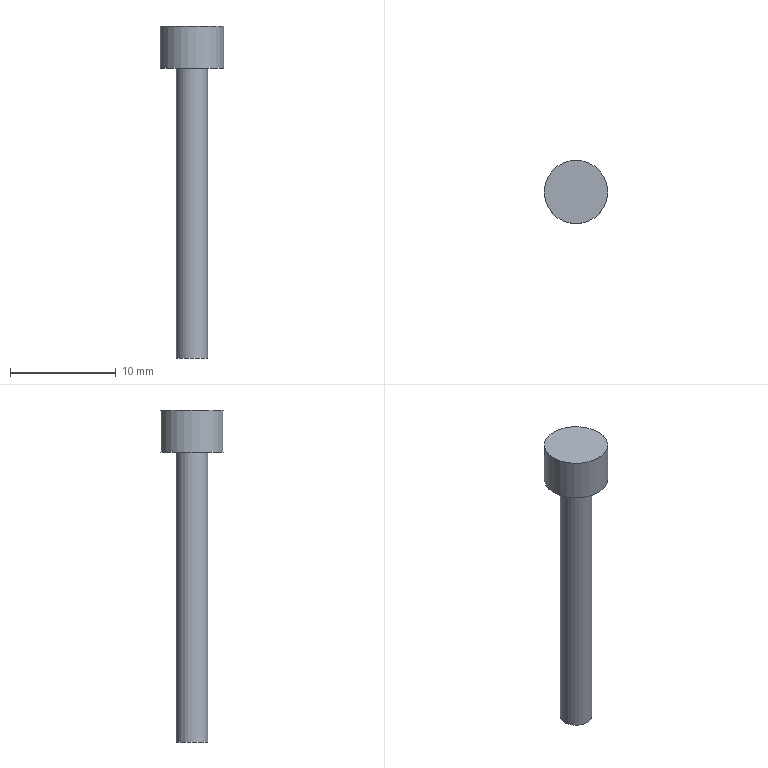Part | STEP file | 1 solid | 5 faces | box 6 x 6 x 31.4 mm | volume 306.777 mm3 | plane 3 | cylinder 2 | commonest cylinder face diameters 3 x1 6 x1
STEP:
#1=CARTESIAN_POINT('',(0.,0.,0.));
#2=DIRECTION('',(0.,0.,1.));
#3=DIRECTION('',(1.,0.,0.));
#4=AXIS2_PLACEMENT_3D('',#1,#2,#3);
#5=CARTESIAN_POINT('',(1482.438,482.48,16.429));
#6=VERTEX_POINT('',#5);
#7=CARTESIAN_POINT('',(1483.938,482.48,16.429));
#8=DIRECTION('',(0.,0.,1.));
#9=DIRECTION('',(-1.,0.,0.));
#10=AXIS2_PLACEMENT_3D('',#7,#8,#9);
#11=CIRCLE('',#10,1.5);
#12=CARTESIAN_POINT('',(1483.938,482.48,16.429));
#13=DIRECTION('',(0.,0.,-1.));
#14=DIRECTION('',(-1.,0.,0.));
#15=AXIS2_PLACEMENT_3D('',#12,#13,#14);
#16=PLANE('',#15);
#17=CARTESIAN_POINT('',(1.5,0.));
#18=CARTESIAN_POINT('',(1.5,-2.598));
#19=CARTESIAN_POINT('',(-0.75,-1.299));
#20=CARTESIAN_POINT('',(-3.,0.));
#21=CARTESIAN_POINT('',(-0.75,1.299));
#22=CARTESIAN_POINT('',(1.5,2.598));
#23=CARTESIAN_POINT('',(1.5,0.));
#24=(BOUNDED_CURVE()B_SPLINE_CURVE(2,(#17,#18,#19,#20,#21,#22,#23),.UNSPECIFIED.,.T.,.F.)B_SPLINE_CURVE_WITH_KNOTS((1,2,2,2,2,1),(-2.094,0.,2.094,4.189,6.283,8.378),.UNSPECIFIED.)CURVE()GEOMETRIC_REPRESENTATION_ITEM()RATIONAL_B_SPLINE_CURVE((1.,0.5,1.,0.5,1.,0.5,1.))REPRESENTATION_ITEM(''));
#25=(GEOMETRIC_REPRESENTATION_CONTEXT(2)PARAMETRIC_REPRESENTATION_CONTEXT()REPRESENTATION_CONTEXT('',''));
#26=DEFINITIONAL_REPRESENTATION('',(#24),#25);
#27=PCURVE('',#16,#26);
#28=CARTESIAN_POINT('',(1483.938,482.48,43.629));
#29=DIRECTION('',(0.,0.,-1.));
#30=DIRECTION('',(-1.,0.,0.));
#31=AXIS2_PLACEMENT_3D('',#28,#29,#30);
#32=CYLINDRICAL_SURFACE('',#31,1.5);
#33=CARTESIAN_POINT('',(6.283,27.2));
#34=DIRECTION('',(-1.,0.));
#35=VECTOR('',#34,1.);
#36=LINE('',#33,#35);
#37=(GEOMETRIC_REPRESENTATION_CONTEXT(2)PARAMETRIC_REPRESENTATION_CONTEXT()REPRESENTATION_CONTEXT('',''));
#38=DEFINITIONAL_REPRESENTATION('',(#36),#37);
#39=PCURVE('',#32,#38);
#40=SURFACE_CURVE('',#11,(#27,#39),.PCURVE_S1.);
#41=EDGE_CURVE('',#6,#6,#40,.T.);
#42=ORIENTED_EDGE('',*,*,#41,.F.);
#43=EDGE_LOOP('',(#42));
#44=FACE_BOUND('',#43,.T.);
#45=ADVANCED_FACE('',(#44),#16,.T.);
#46=ORIENTED_EDGE('',*,*,#41,.T.);
#47=CARTESIAN_POINT('',(1482.438,482.48,43.829));
#48=VERTEX_POINT('',#47);
#49=CARTESIAN_POINT('',(1482.438,482.48,43.829));
#50=CARTESIAN_POINT('',(1482.438,482.48,16.429));
#51=B_SPLINE_CURVE_WITH_KNOTS('',1,(#49,#50),.UNSPECIFIED.,.F.,.F.,(2,2),(-0.2,27.2),.PIECEWISE_BEZIER_KNOTS.);
#52=CARTESIAN_POINT('',(0.,0.));
#53=DIRECTION('',(0.,1.));
#54=VECTOR('',#53,1.);
#55=LINE('',#52,#54);
#56=(GEOMETRIC_REPRESENTATION_CONTEXT(2)PARAMETRIC_REPRESENTATION_CONTEXT()REPRESENTATION_CONTEXT('',''));
#57=DEFINITIONAL_REPRESENTATION('',(#55),#56);
#58=PCURVE('',#32,#57);
#59=CARTESIAN_POINT('',(6.283,0.));
#60=DIRECTION('',(0.,1.));
#61=VECTOR('',#60,1.);
#62=LINE('',#59,#61);
#63=(GEOMETRIC_REPRESENTATION_CONTEXT(2)PARAMETRIC_REPRESENTATION_CONTEXT()REPRESENTATION_CONTEXT('',''));
#64=DEFINITIONAL_REPRESENTATION('',(#62),#63);
#65=PCURVE('',#32,#64);
#66=SEAM_CURVE('',#51,(#58,#65),.PCURVE_S1.);
#67=EDGE_CURVE('',#48,#6,#66,.T.);
#68=ORIENTED_EDGE('',*,*,#67,.F.);
#69=CARTESIAN_POINT('',(1485.438,482.48,43.829));
#70=VERTEX_POINT('',#69);
#71=CARTESIAN_POINT('',(1483.938,482.48,43.829));
#72=DIRECTION('',(0.,0.,1.));
#73=DIRECTION('',(1.,0.,0.));
#74=AXIS2_PLACEMENT_3D('',#71,#72,#73);
#75=CIRCLE('',#74,1.5);
#76=CARTESIAN_POINT('',(3.142,-0.2));
#77=DIRECTION('',(-1.,0.));
#78=VECTOR('',#77,1.);
#79=LINE('',#76,#78);
#80=(GEOMETRIC_REPRESENTATION_CONTEXT(2)PARAMETRIC_REPRESENTATION_CONTEXT()REPRESENTATION_CONTEXT('',''));
#81=DEFINITIONAL_REPRESENTATION('',(#79),#80);
#82=PCURVE('',#32,#81);
#83=CARTESIAN_POINT('',(1483.938,482.48,43.829));
#84=DIRECTION('',(0.,0.,-1.));
#85=DIRECTION('',(-1.,0.,0.));
#86=AXIS2_PLACEMENT_3D('',#83,#84,#85);
#87=PLANE('',#86);
#88=CARTESIAN_POINT('',(-1.5,0.));
#89=CARTESIAN_POINT('',(-1.5,2.598));
#90=CARTESIAN_POINT('',(0.75,1.299));
#91=CARTESIAN_POINT('',(3.,0.));
#92=CARTESIAN_POINT('',(0.75,-1.299));
#93=CARTESIAN_POINT('',(-1.5,-2.598));
#94=CARTESIAN_POINT('',(-1.5,0.));
#95=(BOUNDED_CURVE()B_SPLINE_CURVE(2,(#88,#89,#90,#91,#92,#93,#94),.UNSPECIFIED.,.T.,.F.)B_SPLINE_CURVE_WITH_KNOTS((1,2,2,2,2,1),(-2.094,0.,2.094,4.189,6.283,8.378),.UNSPECIFIED.)CURVE()GEOMETRIC_REPRESENTATION_ITEM()RATIONAL_B_SPLINE_CURVE((1.,0.5,1.,0.5,1.,0.5,1.))REPRESENTATION_ITEM(''));
#96=(GEOMETRIC_REPRESENTATION_CONTEXT(2)PARAMETRIC_REPRESENTATION_CONTEXT()REPRESENTATION_CONTEXT('',''));
#97=DEFINITIONAL_REPRESENTATION('',(#95),#96);
#98=PCURVE('',#87,#97);
#99=SURFACE_CURVE('',#75,(#82,#98),.PCURVE_S1.);
#100=EDGE_CURVE('',#70,#48,#99,.T.);
#101=ORIENTED_EDGE('',*,*,#100,.F.);
#102=CARTESIAN_POINT('',(1483.938,482.48,43.829));
#103=DIRECTION('',(0.,0.,1.));
#104=DIRECTION('',(1.,0.,0.));
#105=AXIS2_PLACEMENT_3D('',#102,#103,#104);
#106=CIRCLE('',#105,1.5);
#107=CARTESIAN_POINT('',(9.425,-0.2));
#108=DIRECTION('',(-1.,0.));
#109=VECTOR('',#108,1.);
#110=LINE('',#107,#109);
#111=(GEOMETRIC_REPRESENTATION_CONTEXT(2)PARAMETRIC_REPRESENTATION_CONTEXT()REPRESENTATION_CONTEXT('',''));
#112=DEFINITIONAL_REPRESENTATION('',(#110),#111);
#113=PCURVE('',#32,#112);
#114=CARTESIAN_POINT('',(-1.5,0.));
#115=CARTESIAN_POINT('',(-1.5,2.598));
#116=CARTESIAN_POINT('',(0.75,1.299));
#117=CARTESIAN_POINT('',(3.,0.));
#118=CARTESIAN_POINT('',(0.75,-1.299));
#119=CARTESIAN_POINT('',(-1.5,-2.598));
#120=CARTESIAN_POINT('',(-1.5,0.));
#121=(BOUNDED_CURVE()B_SPLINE_CURVE(2,(#114,#115,#116,#117,#118,#119,#120),.UNSPECIFIED.,.T.,.F.)B_SPLINE_CURVE_WITH_KNOTS((1,2,2,2,2,1),(-2.094,0.,2.094,4.189,6.283,8.378),.UNSPECIFIED.)CURVE()GEOMETRIC_REPRESENTATION_ITEM()RATIONAL_B_SPLINE_CURVE((1.,0.5,1.,0.5,1.,0.5,1.))REPRESENTATION_ITEM(''));
#122=(GEOMETRIC_REPRESENTATION_CONTEXT(2)PARAMETRIC_REPRESENTATION_CONTEXT()REPRESENTATION_CONTEXT('',''));
#123=DEFINITIONAL_REPRESENTATION('',(#121),#122);
#124=PCURVE('',#87,#123);
#125=SURFACE_CURVE('',#106,(#113,#124),.PCURVE_S1.);
#126=EDGE_CURVE('',#48,#70,#125,.T.);
#127=ORIENTED_EDGE('',*,*,#126,.F.);
#128=ORIENTED_EDGE('',*,*,#67,.T.);
#129=EDGE_LOOP('',(#46,#68,#101,#127,#128));
#130=FACE_BOUND('',#129,.T.);
#131=ADVANCED_FACE('',(#130),#32,.T.);
#132=CARTESIAN_POINT('',(1480.938,482.48,47.829));
#133=VERTEX_POINT('',#132);
#134=CARTESIAN_POINT('',(1483.938,482.48,47.829));
#135=DIRECTION('',(0.,0.,-1.));
#136=DIRECTION('',(-1.,0.,0.));
#137=AXIS2_PLACEMENT_3D('',#134,#135,#136);
#138=CIRCLE('',#137,3.);
#139=CARTESIAN_POINT('',(1483.938,482.48,47.829));
#140=DIRECTION('',(0.,0.,1.));
#141=DIRECTION('',(1.,0.,0.));
#142=AXIS2_PLACEMENT_3D('',#139,#140,#141);
#143=PLANE('',#142);
#144=CARTESIAN_POINT('',(-3.,0.));
#145=CARTESIAN_POINT('',(-3.,5.196));
#146=CARTESIAN_POINT('',(1.5,2.598));
#147=CARTESIAN_POINT('',(6.,0.));
#148=CARTESIAN_POINT('',(1.5,-2.598));
#149=CARTESIAN_POINT('',(-3.,-5.196));
#150=CARTESIAN_POINT('',(-3.,0.));
#151=(BOUNDED_CURVE()B_SPLINE_CURVE(2,(#144,#145,#146,#147,#148,#149,#150),.UNSPECIFIED.,.T.,.F.)B_SPLINE_CURVE_WITH_KNOTS((1,2,2,2,2,1),(-2.094,0.,2.094,4.189,6.283,8.378),.UNSPECIFIED.)CURVE()GEOMETRIC_REPRESENTATION_ITEM()RATIONAL_B_SPLINE_CURVE((1.,0.5,1.,0.5,1.,0.5,1.))REPRESENTATION_ITEM(''));
#152=(GEOMETRIC_REPRESENTATION_CONTEXT(2)PARAMETRIC_REPRESENTATION_CONTEXT()REPRESENTATION_CONTEXT('',''));
#153=DEFINITIONAL_REPRESENTATION('',(#151),#152);
#154=PCURVE('',#143,#153);
#155=CARTESIAN_POINT('',(1483.938,482.48,43.829));
#156=DIRECTION('',(0.,0.,1.));
#157=DIRECTION('',(-1.,0.,0.));
#158=AXIS2_PLACEMENT_3D('',#155,#156,#157);
#159=CYLINDRICAL_SURFACE('',#158,3.);
#160=CARTESIAN_POINT('',(6.283,4.));
#161=DIRECTION('',(-1.,0.));
#162=VECTOR('',#161,1.);
#163=LINE('',#160,#162);
#164=(GEOMETRIC_REPRESENTATION_CONTEXT(2)PARAMETRIC_REPRESENTATION_CONTEXT()REPRESENTATION_CONTEXT('',''));
#165=DEFINITIONAL_REPRESENTATION('',(#163),#164);
#166=PCURVE('',#159,#165);
#167=SURFACE_CURVE('',#138,(#154,#166),.PCURVE_S1.);
#168=EDGE_CURVE('',#133,#133,#167,.T.);
#169=ORIENTED_EDGE('',*,*,#168,.F.);
#170=EDGE_LOOP('',(#169));
#171=FACE_BOUND('',#170,.T.);
#172=ADVANCED_FACE('',(#171),#143,.T.);
#173=ORIENTED_EDGE('',*,*,#100,.T.);
#174=ORIENTED_EDGE('',*,*,#126,.T.);
#175=EDGE_LOOP('',(#173,#174));
#176=FACE_BOUND('',#175,.T.);
#177=CARTESIAN_POINT('',(1486.938,482.48,43.829));
#178=VERTEX_POINT('',#177);
#179=CARTESIAN_POINT('',(1480.938,482.48,43.829));
#180=VERTEX_POINT('',#179);
#181=CARTESIAN_POINT('',(1483.938,482.48,43.829));
#182=DIRECTION('',(0.,0.,1.));
#183=DIRECTION('',(1.,0.,0.));
#184=AXIS2_PLACEMENT_3D('',#181,#182,#183);
#185=CIRCLE('',#184,3.);
#186=CARTESIAN_POINT('',(-3.,0.));
#187=CARTESIAN_POINT('',(-3.,5.196));
#188=CARTESIAN_POINT('',(1.5,2.598));
#189=CARTESIAN_POINT('',(6.,0.));
#190=CARTESIAN_POINT('',(1.5,-2.598));
#191=CARTESIAN_POINT('',(-3.,-5.196));
#192=CARTESIAN_POINT('',(-3.,0.));
#193=(BOUNDED_CURVE()B_SPLINE_CURVE(2,(#186,#187,#188,#189,#190,#191,#192),.UNSPECIFIED.,.T.,.F.)B_SPLINE_CURVE_WITH_KNOTS((1,2,2,2,2,1),(-2.094,0.,2.094,4.189,6.283,8.378),.UNSPECIFIED.)CURVE()GEOMETRIC_REPRESENTATION_ITEM()RATIONAL_B_SPLINE_CURVE((1.,0.5,1.,0.5,1.,0.5,1.))REPRESENTATION_ITEM(''));
#194=(GEOMETRIC_REPRESENTATION_CONTEXT(2)PARAMETRIC_REPRESENTATION_CONTEXT()REPRESENTATION_CONTEXT('',''));
#195=DEFINITIONAL_REPRESENTATION('',(#193),#194);
#196=PCURVE('',#87,#195);
#197=CARTESIAN_POINT('',(3.142,0.));
#198=DIRECTION('',(1.,0.));
#199=VECTOR('',#198,1.);
#200=LINE('',#197,#199);
#201=(GEOMETRIC_REPRESENTATION_CONTEXT(2)PARAMETRIC_REPRESENTATION_CONTEXT()REPRESENTATION_CONTEXT('',''));
#202=DEFINITIONAL_REPRESENTATION('',(#200),#201);
#203=PCURVE('',#159,#202);
#204=SURFACE_CURVE('',#185,(#196,#203),.PCURVE_S1.);
#205=EDGE_CURVE('',#178,#180,#204,.T.);
#206=ORIENTED_EDGE('',*,*,#205,.F.);
#207=CARTESIAN_POINT('',(1483.938,482.48,43.829));
#208=DIRECTION('',(0.,0.,1.));
#209=DIRECTION('',(1.,0.,0.));
#210=AXIS2_PLACEMENT_3D('',#207,#208,#209);
#211=CIRCLE('',#210,3.);
#212=CARTESIAN_POINT('',(-3.,0.));
#213=CARTESIAN_POINT('',(-3.,5.196));
#214=CARTESIAN_POINT('',(1.5,2.598));
#215=CARTESIAN_POINT('',(6.,0.));
#216=CARTESIAN_POINT('',(1.5,-2.598));
#217=CARTESIAN_POINT('',(-3.,-5.196));
#218=CARTESIAN_POINT('',(-3.,0.));
#219=(BOUNDED_CURVE()B_SPLINE_CURVE(2,(#212,#213,#214,#215,#216,#217,#218),.UNSPECIFIED.,.T.,.F.)B_SPLINE_CURVE_WITH_KNOTS((1,2,2,2,2,1),(-2.094,0.,2.094,4.189,6.283,8.378),.UNSPECIFIED.)CURVE()GEOMETRIC_REPRESENTATION_ITEM()RATIONAL_B_SPLINE_CURVE((1.,0.5,1.,0.5,1.,0.5,1.))REPRESENTATION_ITEM(''));
#220=(GEOMETRIC_REPRESENTATION_CONTEXT(2)PARAMETRIC_REPRESENTATION_CONTEXT()REPRESENTATION_CONTEXT('',''));
#221=DEFINITIONAL_REPRESENTATION('',(#219),#220);
#222=PCURVE('',#87,#221);
#223=CARTESIAN_POINT('',(-3.142,0.));
#224=DIRECTION('',(1.,0.));
#225=VECTOR('',#224,1.);
#226=LINE('',#223,#225);
#227=(GEOMETRIC_REPRESENTATION_CONTEXT(2)PARAMETRIC_REPRESENTATION_CONTEXT()REPRESENTATION_CONTEXT('',''));
#228=DEFINITIONAL_REPRESENTATION('',(#226),#227);
#229=PCURVE('',#159,#228);
#230=SURFACE_CURVE('',#211,(#222,#229),.PCURVE_S1.);
#231=EDGE_CURVE('',#180,#178,#230,.T.);
#232=ORIENTED_EDGE('',*,*,#231,.F.);
#233=EDGE_LOOP('',(#206,#232));
#234=FACE_BOUND('',#233,.T.);
#235=ADVANCED_FACE('',(#176,#234),#87,.T.);
#236=ORIENTED_EDGE('',*,*,#168,.T.);
#237=CARTESIAN_POINT('',(1480.938,482.48,43.829));
#238=CARTESIAN_POINT('',(1480.938,482.48,47.829));
#239=B_SPLINE_CURVE_WITH_KNOTS('',1,(#237,#238),.UNSPECIFIED.,.F.,.F.,(2,2),(0.,4.),.PIECEWISE_BEZIER_KNOTS.);
#240=CARTESIAN_POINT('',(0.,0.));
#241=DIRECTION('',(0.,1.));
#242=VECTOR('',#241,1.);
#243=LINE('',#240,#242);
#244=(GEOMETRIC_REPRESENTATION_CONTEXT(2)PARAMETRIC_REPRESENTATION_CONTEXT()REPRESENTATION_CONTEXT('',''));
#245=DEFINITIONAL_REPRESENTATION('',(#243),#244);
#246=PCURVE('',#159,#245);
#247=CARTESIAN_POINT('',(6.283,0.));
#248=DIRECTION('',(0.,1.));
#249=VECTOR('',#248,1.);
#250=LINE('',#247,#249);
#251=(GEOMETRIC_REPRESENTATION_CONTEXT(2)PARAMETRIC_REPRESENTATION_CONTEXT()REPRESENTATION_CONTEXT('',''));
#252=DEFINITIONAL_REPRESENTATION('',(#250),#251);
#253=PCURVE('',#159,#252);
#254=SEAM_CURVE('',#239,(#246,#253),.PCURVE_S1.);
#255=EDGE_CURVE('',#180,#133,#254,.T.);
#256=ORIENTED_EDGE('',*,*,#255,.F.);
#257=ORIENTED_EDGE('',*,*,#231,.T.);
#258=ORIENTED_EDGE('',*,*,#205,.T.);
#259=ORIENTED_EDGE('',*,*,#255,.T.);
#260=EDGE_LOOP('',(#236,#256,#257,#258,#259));
#261=FACE_BOUND('',#260,.T.);
#262=ADVANCED_FACE('',(#261),#159,.T.);
#263=CLOSED_SHELL('',(#45,#131,#172,#235,#262));
#264=MANIFOLD_SOLID_BREP('',#263);
#265=(LENGTH_UNIT()NAMED_UNIT(*)SI_UNIT(.MILLI.,.METRE.));
#266=UNCERTAINTY_MEASURE_WITH_UNIT(LENGTH_MEASURE(0.000005),#265,'','');
#267=(NAMED_UNIT(*)PLANE_ANGLE_UNIT()SI_UNIT($,.RADIAN.));
#268=(NAMED_UNIT(*)SI_UNIT($,.STERADIAN.)SOLID_ANGLE_UNIT());
#269=(GEOMETRIC_REPRESENTATION_CONTEXT(3)GLOBAL_UNCERTAINTY_ASSIGNED_CONTEXT((#266))GLOBAL_UNIT_ASSIGNED_CONTEXT((#265,#267,#268))REPRESENTATION_CONTEXT('',''));
#270=ADVANCED_BREP_SHAPE_REPRESENTATION('',(#4,#264),#269);